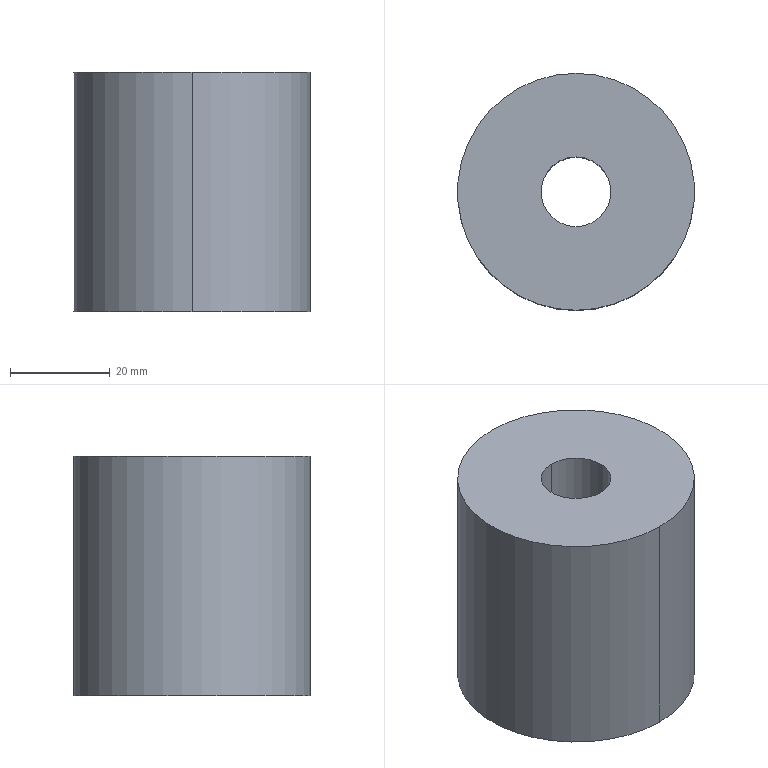Part | SolidWorks | features BaseBody 1 | 1 solid | 6 faces | box 47.5 x 47.5 x 48 mm | volume 77670 mm3 | cylinder 4 | plane 2 | commonest cylinder face diameters 14 x2 47.5 x2
STEP:
#1=CARTESIAN_POINT('',(0.,23.75,0.));
#2=VERTEX_POINT('',#1);
#3=CARTESIAN_POINT('',(0.,-23.75,0.));
#4=VERTEX_POINT('',#3);
#5=CARTESIAN_POINT('',(0.,0.,0.));
#6=DIRECTION('',(0.,0.,-1.));
#7=DIRECTION('',(0.,1.,0.));
#8=AXIS2_PLACEMENT_3D('',#5,#6,#7);
#9=CIRCLE('',#8,23.75);
#10=EDGE_CURVE('',#2,#4,#9,.T.);
#11=ORIENTED_EDGE('',*,*,#10,.T.);
#12=CARTESIAN_POINT('',(0.,-23.75,-48.));
#13=VERTEX_POINT('',#12);
#14=CARTESIAN_POINT('',(0.,-23.75,0.));
#15=DIRECTION('',(0.,0.,-1.));
#16=VECTOR('',#15,1000.);
#17=LINE('',#14,#16);
#18=EDGE_CURVE('',#4,#13,#17,.T.);
#19=ORIENTED_EDGE('',*,*,#18,.T.);
#20=CARTESIAN_POINT('',(0.,23.75,-48.));
#21=VERTEX_POINT('',#20);
#22=CARTESIAN_POINT('',(0.,0.,-48.));
#23=DIRECTION('',(0.,0.,1.));
#24=DIRECTION('',(0.,1.,0.));
#25=AXIS2_PLACEMENT_3D('',#22,#23,#24);
#26=CIRCLE('',#25,23.75);
#27=EDGE_CURVE('',#13,#21,#26,.T.);
#28=ORIENTED_EDGE('',*,*,#27,.T.);
#29=CARTESIAN_POINT('',(0.,23.75,0.));
#30=DIRECTION('',(0.,0.,-1.));
#31=VECTOR('',#30,1000.);
#32=LINE('',#29,#31);
#33=EDGE_CURVE('',#2,#21,#32,.T.);
#34=ORIENTED_EDGE('',*,*,#33,.F.);
#35=EDGE_LOOP('',(#11,#19,#28,#34));
#36=FACE_OUTER_BOUND('',#35,.T.);
#37=CARTESIAN_POINT('',(0.,0.,0.));
#38=DIRECTION('',(0.,0.,-1.));
#39=DIRECTION('',(0.,1.,0.));
#40=AXIS2_PLACEMENT_3D('',#37,#38,#39);
#41=CYLINDRICAL_SURFACE('',#40,23.75);
#42=ADVANCED_FACE('',(#36),#41,.T.);
#43=CARTESIAN_POINT('',(0.,-7.,0.));
#44=VERTEX_POINT('',#43);
#45=CARTESIAN_POINT('',(0.,7.,0.));
#46=VERTEX_POINT('',#45);
#47=CARTESIAN_POINT('',(0.,0.,0.));
#48=DIRECTION('',(0.,0.,-1.));
#49=DIRECTION('',(0.,1.,0.));
#50=AXIS2_PLACEMENT_3D('',#47,#48,#49);
#51=CIRCLE('',#50,7.);
#52=EDGE_CURVE('',#44,#46,#51,.T.);
#53=ORIENTED_EDGE('',*,*,#52,.F.);
#54=CARTESIAN_POINT('',(0.,-7.,-48.));
#55=VERTEX_POINT('',#54);
#56=CARTESIAN_POINT('',(0.,-7.,0.));
#57=DIRECTION('',(0.,0.,-1.));
#58=VECTOR('',#57,1000.);
#59=LINE('',#56,#58);
#60=EDGE_CURVE('',#44,#55,#59,.T.);
#61=ORIENTED_EDGE('',*,*,#60,.T.);
#62=CARTESIAN_POINT('',(0.,7.,-48.));
#63=VERTEX_POINT('',#62);
#64=CARTESIAN_POINT('',(0.,0.,-48.));
#65=DIRECTION('',(0.,0.,1.));
#66=DIRECTION('',(0.,1.,0.));
#67=AXIS2_PLACEMENT_3D('',#64,#65,#66);
#68=CIRCLE('',#67,7.);
#69=EDGE_CURVE('',#63,#55,#68,.T.);
#70=ORIENTED_EDGE('',*,*,#69,.F.);
#71=CARTESIAN_POINT('',(0.,7.,0.));
#72=DIRECTION('',(0.,0.,-1.));
#73=VECTOR('',#72,1000.);
#74=LINE('',#71,#73);
#75=EDGE_CURVE('',#46,#63,#74,.T.);
#76=ORIENTED_EDGE('',*,*,#75,.F.);
#77=EDGE_LOOP('',(#53,#61,#70,#76));
#78=FACE_OUTER_BOUND('',#77,.T.);
#79=CARTESIAN_POINT('',(0.,0.,0.));
#80=DIRECTION('',(0.,0.,-1.));
#81=DIRECTION('',(0.,1.,0.));
#82=AXIS2_PLACEMENT_3D('',#79,#80,#81);
#83=CYLINDRICAL_SURFACE('',#82,7.);
#84=ADVANCED_FACE('',(#78),#83,.F.);
#85=ORIENTED_EDGE('',*,*,#18,.F.);
#86=CARTESIAN_POINT('',(0.,0.,0.));
#87=DIRECTION('',(0.,0.,-1.));
#88=DIRECTION('',(0.,1.,0.));
#89=AXIS2_PLACEMENT_3D('',#86,#87,#88);
#90=CIRCLE('',#89,23.75);
#91=EDGE_CURVE('',#4,#2,#90,.T.);
#92=ORIENTED_EDGE('',*,*,#91,.T.);
#93=ORIENTED_EDGE('',*,*,#33,.T.);
#94=CARTESIAN_POINT('',(0.,0.,-48.));
#95=DIRECTION('',(0.,0.,1.));
#96=DIRECTION('',(0.,1.,0.));
#97=AXIS2_PLACEMENT_3D('',#94,#95,#96);
#98=CIRCLE('',#97,23.75);
#99=EDGE_CURVE('',#21,#13,#98,.T.);
#100=ORIENTED_EDGE('',*,*,#99,.T.);
#101=EDGE_LOOP('',(#85,#92,#93,#100));
#102=FACE_OUTER_BOUND('',#101,.T.);
#103=CARTESIAN_POINT('',(0.,0.,0.));
#104=DIRECTION('',(0.,0.,-1.));
#105=DIRECTION('',(0.,1.,0.));
#106=AXIS2_PLACEMENT_3D('',#103,#104,#105);
#107=CYLINDRICAL_SURFACE('',#106,23.75);
#108=ADVANCED_FACE('',(#102),#107,.T.);
#109=ORIENTED_EDGE('',*,*,#69,.T.);
#110=CARTESIAN_POINT('',(0.,0.,-48.));
#111=DIRECTION('',(0.,0.,1.));
#112=DIRECTION('',(0.,1.,0.));
#113=AXIS2_PLACEMENT_3D('',#110,#111,#112);
#114=CIRCLE('',#113,7.);
#115=EDGE_CURVE('',#55,#63,#114,.T.);
#116=ORIENTED_EDGE('',*,*,#115,.T.);
#117=EDGE_LOOP('',(#109,#116));
#118=FACE_BOUND('',#117,.T.);
#119=ORIENTED_EDGE('',*,*,#99,.F.);
#120=ORIENTED_EDGE('',*,*,#27,.F.);
#121=EDGE_LOOP('',(#119,#120));
#122=FACE_OUTER_BOUND('',#121,.T.);
#123=CARTESIAN_POINT('',(7.,0.,-48.));
#124=DIRECTION('',(0.,0.,-1.));
#125=DIRECTION('',(0.,1.,0.));
#126=AXIS2_PLACEMENT_3D('',#123,#124,#125);
#127=PLANE('',#126);
#128=ADVANCED_FACE('',(#118,#122),#127,.T.);
#129=ORIENTED_EDGE('',*,*,#10,.F.);
#130=ORIENTED_EDGE('',*,*,#91,.F.);
#131=EDGE_LOOP('',(#129,#130));
#132=FACE_OUTER_BOUND('',#131,.T.);
#133=CARTESIAN_POINT('',(0.,0.,0.));
#134=DIRECTION('',(0.,0.,-1.));
#135=DIRECTION('',(0.,1.,0.));
#136=AXIS2_PLACEMENT_3D('',#133,#134,#135);
#137=CIRCLE('',#136,7.);
#138=EDGE_CURVE('',#46,#44,#137,.T.);
#139=ORIENTED_EDGE('',*,*,#138,.T.);
#140=ORIENTED_EDGE('',*,*,#52,.T.);
#141=EDGE_LOOP('',(#139,#140));
#142=FACE_BOUND('',#141,.T.);
#143=CARTESIAN_POINT('',(23.75,0.,0.));
#144=DIRECTION('',(0.,0.,1.));
#145=DIRECTION('',(0.,-1.,0.));
#146=AXIS2_PLACEMENT_3D('',#143,#144,#145);
#147=PLANE('',#146);
#148=ADVANCED_FACE('',(#132,#142),#147,.T.);
#149=ORIENTED_EDGE('',*,*,#60,.F.);
#150=ORIENTED_EDGE('',*,*,#138,.F.);
#151=ORIENTED_EDGE('',*,*,#75,.T.);
#152=ORIENTED_EDGE('',*,*,#115,.F.);
#153=EDGE_LOOP('',(#149,#150,#151,#152));
#154=FACE_OUTER_BOUND('',#153,.T.);
#155=CARTESIAN_POINT('',(0.,0.,0.));
#156=DIRECTION('',(0.,0.,-1.));
#157=DIRECTION('',(0.,1.,0.));
#158=AXIS2_PLACEMENT_3D('',#155,#156,#157);
#159=CYLINDRICAL_SURFACE('',#158,7.);
#160=ADVANCED_FACE('',(#154),#159,.F.);
#161=CLOSED_SHELL('',(#42,#84,#108,#128,#148,#160));
#162=MANIFOLD_SOLID_BREP('',#161);
#163=CARTESIAN_POINT('',(0.,0.,0.));
#164=DIRECTION('',(0.,0.,1.));
#165=DIRECTION('',(1.,0.,0.));
#166=AXIS2_PLACEMENT_3D('',#163,#164,#165);
#167=(LENGTH_UNIT()NAMED_UNIT(*)SI_UNIT(.MILLI.,.METRE.));
#168=UNCERTAINTY_MEASURE_WITH_UNIT(LENGTH_MEASURE(0.00001),#167,'','');
#169=(NAMED_UNIT(*)PLANE_ANGLE_UNIT()SI_UNIT($,.RADIAN.));
#170=(NAMED_UNIT(*)SI_UNIT($,.STERADIAN.)SOLID_ANGLE_UNIT());
#171=(GEOMETRIC_REPRESENTATION_CONTEXT(3)GLOBAL_UNCERTAINTY_ASSIGNED_CONTEXT((#168))GLOBAL_UNIT_ASSIGNED_CONTEXT((#167,#169,#170))REPRESENTATION_CONTEXT('',''));
#172=ADVANCED_BREP_SHAPE_REPRESENTATION('',(#162,#166),#171);